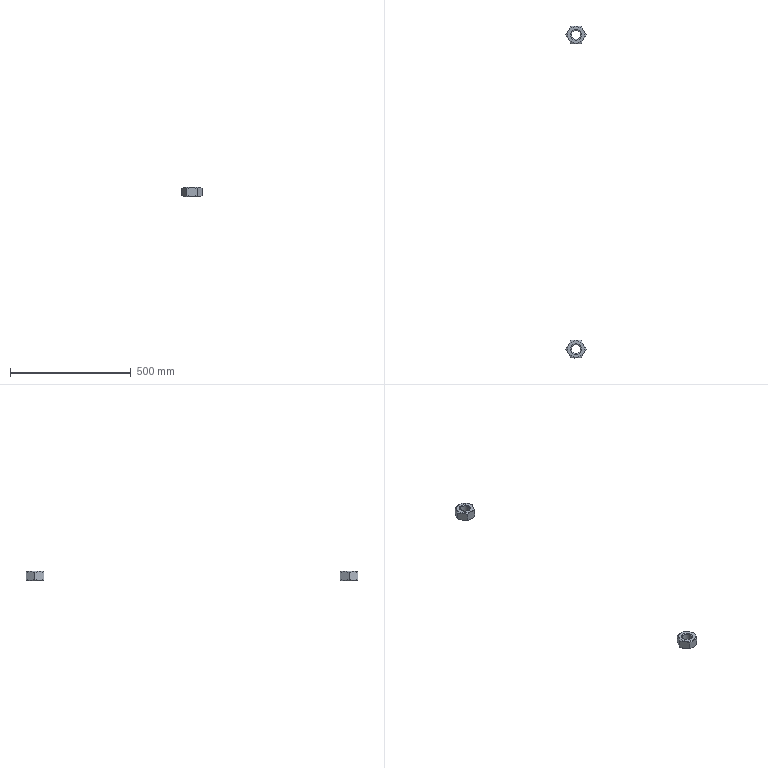Part | NX | features 11.SLDPRT 2, Delete Body 1, LINKED_BODY 1, SCALE 1 | 2 solids | 26 faces | box 84.437 x 1373 x 38.25 mm | volume 263240 mm3 | plane 16 | cone 8 | cylinder 2 | commonest cylinder face diameters 37.389 x2
STEP:
#1=CARTESIAN_POINT('',(28.359,882.042,-396.441));
#2=VERTEX_POINT('',#1);
#3=CARTESIAN_POINT('',(49.469,918.604,-396.441));
#4=VERTEX_POINT('',#3);
#5=CARTESIAN_POINT('',(28.359,882.042,-396.441));
#6=CARTESIAN_POINT('',(30.083,885.027,-395.446));
#7=CARTESIAN_POINT('',(33.551,891.033,-393.805));
#8=CARTESIAN_POINT('',(38.885,900.273,-392.862));
#9=CARTESIAN_POINT('',(44.273,909.605,-393.798));
#10=CARTESIAN_POINT('',(47.743,915.616,-395.445));
#11=CARTESIAN_POINT('',(49.469,918.604,-396.441));
#12=B_SPLINE_CURVE_WITH_KNOTS('',3,(#5,#6,#7,#8,#9,#10,#11),.UNSPECIFIED.,.F.,.F.,(4,1,1,1,4),(0.000001339,0.01066,0.02132,0.03198,0.04264),.UNSPECIFIED.);
#13=EDGE_CURVE('',#2,#4,#12,.T.);
#14=ORIENTED_EDGE('',*,*,#13,.F.);
#15=CARTESIAN_POINT('',(28.359,882.042,-425.724));
#16=VERTEX_POINT('',#15);
#17=CARTESIAN_POINT('',(28.359,882.042,-430.207));
#18=DIRECTION('',(0.,0.,1.));
#19=VECTOR('',#18,1000.);
#20=LINE('',#17,#19);
#21=EDGE_CURVE('',#16,#2,#20,.T.);
#22=ORIENTED_EDGE('',*,*,#21,.F.);
#23=CARTESIAN_POINT('',(49.469,918.604,-425.724));
#24=VERTEX_POINT('',#23);
#25=CARTESIAN_POINT('',(49.469,918.604,-425.724));
#26=CARTESIAN_POINT('',(47.745,915.619,-426.719));
#27=CARTESIAN_POINT('',(44.277,909.613,-428.36));
#28=CARTESIAN_POINT('',(38.943,900.373,-429.303));
#29=CARTESIAN_POINT('',(33.555,891.042,-428.367));
#30=CARTESIAN_POINT('',(30.085,885.031,-426.72));
#31=CARTESIAN_POINT('',(28.359,882.042,-425.724));
#32=B_SPLINE_CURVE_WITH_KNOTS('',3,(#25,#26,#27,#28,#29,#30,#31),.UNSPECIFIED.,.F.,.F.,(4,1,1,1,4),(0.000001339,0.01066,0.02132,0.03198,0.04264),.UNSPECIFIED.);
#33=EDGE_CURVE('',#24,#16,#32,.T.);
#34=ORIENTED_EDGE('',*,*,#33,.F.);
#35=CARTESIAN_POINT('',(49.469,918.604,-430.207));
#36=DIRECTION('',(0.,0.,1.));
#37=VECTOR('',#36,1000.);
#38=LINE('',#35,#37);
#39=EDGE_CURVE('',#24,#4,#38,.T.);
#40=ORIENTED_EDGE('',*,*,#39,.T.);
#41=EDGE_LOOP('',(#14,#22,#34,#40));
#42=FACE_BOUND('',#41,.T.);
#43=CARTESIAN_POINT('',(28.359,882.042,-430.207));
#44=DIRECTION('',(0.866,-0.5,0.));
#45=DIRECTION('',(0.5,0.866,0.));
#46=AXIS2_PLACEMENT_3D('',#43,#44,#45);
#47=PLANE('',#46);
#48=ADVANCED_FACE('',(#42),#47,.T.);
#49=CARTESIAN_POINT('',(-13.859,882.042,-396.441));
#50=VERTEX_POINT('',#49);
#51=CARTESIAN_POINT('',(-13.859,882.042,-396.441));
#52=CARTESIAN_POINT('',(-10.426,882.042,-395.45));
#53=CARTESIAN_POINT('',(-3.394,882.042,-393.789));
#54=CARTESIAN_POINT('',(7.222,882.042,-392.864));
#55=CARTESIAN_POINT('',(18.042,882.042,-393.809));
#56=CARTESIAN_POINT('',(24.947,882.042,-395.456));
#57=CARTESIAN_POINT('',(28.359,882.042,-396.441));
#58=B_SPLINE_CURVE_WITH_KNOTS('',3,(#51,#52,#53,#54,#55,#56,#57),.UNSPECIFIED.,.F.,.F.,(4,1,1,1,4),(0.03747,0.04815,0.05883,0.06951,0.08019),.UNSPECIFIED.);
#59=EDGE_CURVE('',#50,#2,#58,.T.);
#60=ORIENTED_EDGE('',*,*,#59,.F.);
#61=CARTESIAN_POINT('',(-13.859,882.042,-425.724));
#62=VERTEX_POINT('',#61);
#63=CARTESIAN_POINT('',(-13.859,882.042,-430.207));
#64=DIRECTION('',(0.,0.,1.));
#65=VECTOR('',#64,1000.);
#66=LINE('',#63,#65);
#67=EDGE_CURVE('',#62,#50,#66,.T.);
#68=ORIENTED_EDGE('',*,*,#67,.F.);
#69=CARTESIAN_POINT('',(-13.859,882.042,-425.724));
#70=CARTESIAN_POINT('',(-10.426,882.042,-426.715));
#71=CARTESIAN_POINT('',(-3.394,882.042,-428.376));
#72=CARTESIAN_POINT('',(7.222,882.042,-429.301));
#73=CARTESIAN_POINT('',(18.042,882.042,-428.356));
#74=CARTESIAN_POINT('',(24.947,882.042,-426.709));
#75=CARTESIAN_POINT('',(28.359,882.042,-425.724));
#76=B_SPLINE_CURVE_WITH_KNOTS('',3,(#69,#70,#71,#72,#73,#74,#75),.UNSPECIFIED.,.F.,.F.,(4,1,1,1,4),(0.03747,0.04815,0.05883,0.06951,0.08019),.UNSPECIFIED.);
#77=EDGE_CURVE('',#16,#62,#76,.F.);
#78=ORIENTED_EDGE('',*,*,#77,.F.);
#79=ORIENTED_EDGE('',*,*,#21,.T.);
#80=EDGE_LOOP('',(#60,#68,#78,#79));
#81=FACE_BOUND('',#80,.T.);
#82=CARTESIAN_POINT('',(-13.859,882.042,-430.207));
#83=DIRECTION('',(0.,-1.,0.));
#84=DIRECTION('',(1.,0.,0.));
#85=AXIS2_PLACEMENT_3D('',#82,#83,#84);
#86=PLANE('',#85);
#87=ADVANCED_FACE('',(#81),#86,.T.);
#88=CARTESIAN_POINT('',(-34.969,918.604,-396.441));
#89=VERTEX_POINT('',#88);
#90=CARTESIAN_POINT('',(-34.969,918.604,-396.441));
#91=CARTESIAN_POINT('',(-33.245,915.619,-395.446));
#92=CARTESIAN_POINT('',(-29.777,909.613,-393.805));
#93=CARTESIAN_POINT('',(-24.443,900.373,-392.862));
#94=CARTESIAN_POINT('',(-19.055,891.042,-393.798));
#95=CARTESIAN_POINT('',(-15.585,885.031,-395.445));
#96=CARTESIAN_POINT('',(-13.859,882.042,-396.441));
#97=B_SPLINE_CURVE_WITH_KNOTS('',3,(#90,#91,#92,#93,#94,#95,#96),.UNSPECIFIED.,.F.,.F.,(4,1,1,1,4),(0.000001339,0.01066,0.02132,0.03198,0.04264),.UNSPECIFIED.);
#98=EDGE_CURVE('',#89,#50,#97,.T.);
#99=ORIENTED_EDGE('',*,*,#98,.F.);
#100=CARTESIAN_POINT('',(-34.969,918.604,-425.724));
#101=VERTEX_POINT('',#100);
#102=CARTESIAN_POINT('',(-34.969,918.604,-430.207));
#103=DIRECTION('',(0.,0.,1.));
#104=VECTOR('',#103,1000.);
#105=LINE('',#102,#104);
#106=EDGE_CURVE('',#101,#89,#105,.T.);
#107=ORIENTED_EDGE('',*,*,#106,.F.);
#108=CARTESIAN_POINT('',(-13.859,882.042,-425.724));
#109=CARTESIAN_POINT('',(-15.583,885.027,-426.719));
#110=CARTESIAN_POINT('',(-19.051,891.033,-428.36));
#111=CARTESIAN_POINT('',(-24.385,900.273,-429.303));
#112=CARTESIAN_POINT('',(-29.773,909.605,-428.367));
#113=CARTESIAN_POINT('',(-33.243,915.616,-426.72));
#114=CARTESIAN_POINT('',(-34.969,918.604,-425.724));
#115=B_SPLINE_CURVE_WITH_KNOTS('',3,(#108,#109,#110,#111,#112,#113,#114),.UNSPECIFIED.,.F.,.F.,(4,1,1,1,4),(0.000001339,0.01066,0.02132,0.03198,0.04264),.UNSPECIFIED.);
#116=EDGE_CURVE('',#62,#101,#115,.T.);
#117=ORIENTED_EDGE('',*,*,#116,.F.);
#118=ORIENTED_EDGE('',*,*,#67,.T.);
#119=EDGE_LOOP('',(#99,#107,#117,#118));
#120=FACE_BOUND('',#119,.T.);
#121=CARTESIAN_POINT('',(-34.969,918.604,-430.207));
#122=DIRECTION('',(-0.866,-0.5,0.));
#123=DIRECTION('',(0.5,-0.866,0.));
#124=AXIS2_PLACEMENT_3D('',#121,#122,#123);
#125=PLANE('',#124);
#126=ADVANCED_FACE('',(#120),#125,.T.);
#127=CARTESIAN_POINT('',(-13.859,955.167,-396.441));
#128=VERTEX_POINT('',#127);
#129=CARTESIAN_POINT('',(-13.859,955.167,-396.441));
#130=CARTESIAN_POINT('',(-15.583,952.182,-395.446));
#131=CARTESIAN_POINT('',(-19.051,946.175,-393.805));
#132=CARTESIAN_POINT('',(-24.385,936.936,-392.862));
#133=CARTESIAN_POINT('',(-29.773,927.604,-393.798));
#134=CARTESIAN_POINT('',(-33.243,921.593,-395.445));
#135=CARTESIAN_POINT('',(-34.969,918.604,-396.441));
#136=B_SPLINE_CURVE_WITH_KNOTS('',3,(#129,#130,#131,#132,#133,#134,#135),.UNSPECIFIED.,.F.,.F.,(4,1,1,1,4),(0.000001339,0.01066,0.02132,0.03198,0.04264),.UNSPECIFIED.);
#137=EDGE_CURVE('',#128,#89,#136,.T.);
#138=ORIENTED_EDGE('',*,*,#137,.F.);
#139=CARTESIAN_POINT('',(-13.859,955.167,-425.724));
#140=VERTEX_POINT('',#139);
#141=CARTESIAN_POINT('',(-13.859,955.167,-430.207));
#142=DIRECTION('',(0.,0.,1.));
#143=VECTOR('',#142,1000.);
#144=LINE('',#141,#143);
#145=EDGE_CURVE('',#140,#128,#144,.T.);
#146=ORIENTED_EDGE('',*,*,#145,.F.);
#147=CARTESIAN_POINT('',(-34.969,918.604,-425.724));
#148=CARTESIAN_POINT('',(-33.245,921.589,-426.719));
#149=CARTESIAN_POINT('',(-29.777,927.596,-428.36));
#150=CARTESIAN_POINT('',(-24.443,936.835,-429.303));
#151=CARTESIAN_POINT('',(-19.055,946.167,-428.367));
#152=CARTESIAN_POINT('',(-15.585,952.178,-426.72));
#153=CARTESIAN_POINT('',(-13.859,955.167,-425.724));
#154=B_SPLINE_CURVE_WITH_KNOTS('',3,(#147,#148,#149,#150,#151,#152,#153),.UNSPECIFIED.,.F.,.F.,(4,1,1,1,4),(0.000001339,0.01066,0.02132,0.03198,0.04264),.UNSPECIFIED.);
#155=EDGE_CURVE('',#101,#140,#154,.T.);
#156=ORIENTED_EDGE('',*,*,#155,.F.);
#157=ORIENTED_EDGE('',*,*,#106,.T.);
#158=EDGE_LOOP('',(#138,#146,#156,#157));
#159=FACE_BOUND('',#158,.T.);
#160=CARTESIAN_POINT('',(-13.859,955.167,-430.207));
#161=DIRECTION('',(-0.866,0.5,0.));
#162=DIRECTION('',(-0.5,-0.866,0.));
#163=AXIS2_PLACEMENT_3D('',#160,#161,#162);
#164=PLANE('',#163);
#165=ADVANCED_FACE('',(#159),#164,.T.);
#166=CARTESIAN_POINT('',(28.359,955.167,-396.441));
#167=VERTEX_POINT('',#166);
#168=CARTESIAN_POINT('',(-13.859,955.167,-396.441));
#169=CARTESIAN_POINT('',(-10.426,955.167,-395.45));
#170=CARTESIAN_POINT('',(-3.394,955.167,-393.789));
#171=CARTESIAN_POINT('',(7.222,955.167,-392.864));
#172=CARTESIAN_POINT('',(18.042,955.167,-393.809));
#173=CARTESIAN_POINT('',(24.947,955.167,-395.456));
#174=CARTESIAN_POINT('',(28.359,955.167,-396.441));
#175=B_SPLINE_CURVE_WITH_KNOTS('',3,(#168,#169,#170,#171,#172,#173,#174),.UNSPECIFIED.,.F.,.F.,(4,1,1,1,4),(0.03747,0.04815,0.05883,0.06951,0.08019),.UNSPECIFIED.);
#176=EDGE_CURVE('',#167,#128,#175,.F.);
#177=ORIENTED_EDGE('',*,*,#176,.F.);
#178=CARTESIAN_POINT('',(28.359,955.167,-425.724));
#179=VERTEX_POINT('',#178);
#180=CARTESIAN_POINT('',(28.359,955.167,-430.207));
#181=DIRECTION('',(0.,0.,1.));
#182=VECTOR('',#181,1000.);
#183=LINE('',#180,#182);
#184=EDGE_CURVE('',#179,#167,#183,.T.);
#185=ORIENTED_EDGE('',*,*,#184,.F.);
#186=CARTESIAN_POINT('',(-13.859,955.167,-425.724));
#187=CARTESIAN_POINT('',(-10.426,955.167,-426.715));
#188=CARTESIAN_POINT('',(-3.394,955.167,-428.376));
#189=CARTESIAN_POINT('',(7.222,955.167,-429.301));
#190=CARTESIAN_POINT('',(18.042,955.167,-428.356));
#191=CARTESIAN_POINT('',(24.947,955.167,-426.709));
#192=CARTESIAN_POINT('',(28.359,955.167,-425.724));
#193=B_SPLINE_CURVE_WITH_KNOTS('',3,(#186,#187,#188,#189,#190,#191,#192),.UNSPECIFIED.,.F.,.F.,(4,1,1,1,4),(0.03747,0.04815,0.05883,0.06951,0.08019),.UNSPECIFIED.);
#194=EDGE_CURVE('',#140,#179,#193,.T.);
#195=ORIENTED_EDGE('',*,*,#194,.F.);
#196=ORIENTED_EDGE('',*,*,#145,.T.);
#197=EDGE_LOOP('',(#177,#185,#195,#196));
#198=FACE_BOUND('',#197,.T.);
#199=CARTESIAN_POINT('',(28.359,955.167,-430.207));
#200=DIRECTION('',(0.,1.,0.));
#201=DIRECTION('',(0.,0.,1.));
#202=AXIS2_PLACEMENT_3D('',#199,#200,#201);
#203=PLANE('',#202);
#204=ADVANCED_FACE('',(#198),#203,.T.);
#205=CARTESIAN_POINT('',(49.469,918.604,-396.441));
#206=CARTESIAN_POINT('',(47.745,921.589,-395.446));
#207=CARTESIAN_POINT('',(44.277,927.596,-393.805));
#208=CARTESIAN_POINT('',(38.943,936.835,-392.862));
#209=CARTESIAN_POINT('',(33.555,946.167,-393.798));
#210=CARTESIAN_POINT('',(30.085,952.178,-395.445));
#211=CARTESIAN_POINT('',(28.359,955.167,-396.441));
#212=B_SPLINE_CURVE_WITH_KNOTS('',3,(#205,#206,#207,#208,#209,#210,#211),.UNSPECIFIED.,.F.,.F.,(4,1,1,1,4),(0.000001339,0.01066,0.02132,0.03198,0.04264),.UNSPECIFIED.);
#213=EDGE_CURVE('',#4,#167,#212,.T.);
#214=ORIENTED_EDGE('',*,*,#213,.F.);
#215=ORIENTED_EDGE('',*,*,#39,.F.);
#216=CARTESIAN_POINT('',(28.359,955.167,-425.724));
#217=CARTESIAN_POINT('',(30.083,952.182,-426.719));
#218=CARTESIAN_POINT('',(33.551,946.175,-428.36));
#219=CARTESIAN_POINT('',(38.885,936.936,-429.303));
#220=CARTESIAN_POINT('',(44.273,927.604,-428.367));
#221=CARTESIAN_POINT('',(47.743,921.593,-426.72));
#222=CARTESIAN_POINT('',(49.469,918.604,-425.724));
#223=B_SPLINE_CURVE_WITH_KNOTS('',3,(#216,#217,#218,#219,#220,#221,#222),.UNSPECIFIED.,.F.,.F.,(4,1,1,1,4),(0.000001339,0.01066,0.02132,0.03198,0.04264),.UNSPECIFIED.);
#224=EDGE_CURVE('',#179,#24,#223,.T.);
#225=ORIENTED_EDGE('',*,*,#224,.F.);
#226=ORIENTED_EDGE('',*,*,#184,.T.);
#227=EDGE_LOOP('',(#214,#215,#225,#226));
#228=FACE_BOUND('',#227,.T.);
#229=CARTESIAN_POINT('',(49.469,918.604,-430.207));
#230=DIRECTION('',(0.866,0.5,0.));
#231=DIRECTION('',(-0.5,0.866,0.));
#232=AXIS2_PLACEMENT_3D('',#229,#230,#231);
#233=PLANE('',#232);
#234=ADVANCED_FACE('',(#228),#233,.T.);
#235=CARTESIAN_POINT('',(28.142,918.604,-430.207));
#236=VERTEX_POINT('',#235);
#237=CARTESIAN_POINT('',(7.25,918.604,-430.207));
#238=DIRECTION('',(0.,0.,1.));
#239=DIRECTION('',(1.,0.,0.));
#240=AXIS2_PLACEMENT_3D('',#237,#238,#239);
#241=CIRCLE('',#240,20.892);
#242=EDGE_CURVE('',#236,#236,#241,.T.);
#243=ORIENTED_EDGE('',*,*,#242,.T.);
#244=EDGE_LOOP('',(#243));
#245=FACE_BOUND('',#244,.T.);
#246=CARTESIAN_POINT('',(-27.203,918.604,-430.207));
#247=VERTEX_POINT('',#246);
#248=CARTESIAN_POINT('',(7.25,918.604,-430.207));
#249=DIRECTION('',(0.,0.,-1.));
#250=DIRECTION('',(-1.,0.,0.));
#251=AXIS2_PLACEMENT_3D('',#248,#249,#250);
#252=CIRCLE('',#251,34.453);
#253=EDGE_CURVE('',#247,#247,#252,.T.);
#254=ORIENTED_EDGE('',*,*,#253,.T.);
#255=EDGE_LOOP('',(#254));
#256=FACE_BOUND('',#255,.T.);
#257=CARTESIAN_POINT('',(49.469,918.604,-430.207));
#258=DIRECTION('',(0.,0.,1.));
#259=DIRECTION('',(1.,0.,0.));
#260=AXIS2_PLACEMENT_3D('',#257,#258,#259);
#261=PLANE('',#260);
#262=ADVANCED_FACE('',(#245,#256),#261,.F.);
#263=CARTESIAN_POINT('',(29.75,918.604,-391.957));
#264=VERTEX_POINT('',#263);
#265=CARTESIAN_POINT('',(7.25,918.604,-391.957));
#266=DIRECTION('',(0.,0.,1.));
#267=DIRECTION('',(1.,0.,0.));
#268=AXIS2_PLACEMENT_3D('',#265,#266,#267);
#269=CIRCLE('',#268,22.5);
#270=EDGE_CURVE('',#264,#264,#269,.F.);
#271=ORIENTED_EDGE('',*,*,#270,.T.);
#272=EDGE_LOOP('',(#271));
#273=FACE_BOUND('',#272,.T.);
#274=CARTESIAN_POINT('',(-27.203,918.604,-391.957));
#275=VERTEX_POINT('',#274);
#276=CARTESIAN_POINT('',(7.25,918.604,-391.957));
#277=DIRECTION('',(0.,0.,-1.));
#278=DIRECTION('',(-1.,0.,0.));
#279=AXIS2_PLACEMENT_3D('',#276,#277,#278);
#280=CIRCLE('',#279,34.453);
#281=EDGE_CURVE('',#275,#275,#280,.T.);
#282=ORIENTED_EDGE('',*,*,#281,.F.);
#283=EDGE_LOOP('',(#282));
#284=FACE_BOUND('',#283,.T.);
#285=CARTESIAN_POINT('',(49.469,918.604,-391.957));
#286=DIRECTION('',(0.,0.,1.));
#287=DIRECTION('',(1.,0.,0.));
#288=AXIS2_PLACEMENT_3D('',#285,#286,#287);
#289=PLANE('',#288);
#290=ADVANCED_FACE('',(#273,#284),#289,.T.);
#291=CARTESIAN_POINT('',(25.945,918.604,-426.402));
#292=VERTEX_POINT('',#291);
#293=CARTESIAN_POINT('',(7.25,918.604,-426.402));
#294=DIRECTION('',(0.,0.,1.));
#295=DIRECTION('',(1.,0.,0.));
#296=AXIS2_PLACEMENT_3D('',#293,#294,#295);
#297=CIRCLE('',#296,18.695);
#298=EDGE_CURVE('',#292,#292,#297,.F.);
#299=ORIENTED_EDGE('',*,*,#298,.T.);
#300=EDGE_LOOP('',(#299));
#301=FACE_BOUND('',#300,.T.);
#302=CARTESIAN_POINT('',(25.945,918.604,-394.154));
#303=VERTEX_POINT('',#302);
#304=CARTESIAN_POINT('',(7.25,918.604,-394.154));
#305=DIRECTION('',(0.,0.,1.));
#306=DIRECTION('',(1.,0.,0.));
#307=AXIS2_PLACEMENT_3D('',#304,#305,#306);
#308=CIRCLE('',#307,18.695);
#309=EDGE_CURVE('',#303,#303,#308,.T.);
#310=ORIENTED_EDGE('',*,*,#309,.T.);
#311=EDGE_LOOP('',(#310));
#312=FACE_BOUND('',#311,.T.);
#313=CARTESIAN_POINT('',(7.25,918.604,-430.207));
#314=DIRECTION('',(0.,0.,1.));
#315=DIRECTION('',(1.,0.,0.));
#316=AXIS2_PLACEMENT_3D('',#313,#314,#315);
#317=CYLINDRICAL_SURFACE('',#316,18.695);
#318=ADVANCED_FACE('',(#301,#312),#317,.F.);
#319=ORIENTED_EDGE('',*,*,#33,.T.);
#320=ORIENTED_EDGE('',*,*,#77,.T.);
#321=ORIENTED_EDGE('',*,*,#116,.T.);
#322=ORIENTED_EDGE('',*,*,#155,.T.);
#323=ORIENTED_EDGE('',*,*,#194,.T.);
#324=ORIENTED_EDGE('',*,*,#224,.T.);
#325=EDGE_LOOP('',(#319,#320,#321,#322,#323,#324));
#326=FACE_BOUND('',#325,.T.);
#327=ORIENTED_EDGE('',*,*,#253,.F.);
#328=EDGE_LOOP('',(#327));
#329=FACE_BOUND('',#328,.T.);
#330=CARTESIAN_POINT('',(7.25,918.604,-425.724));
#331=DIRECTION('',(0.,0.,1.));
#332=DIRECTION('',(1.,0.,0.));
#333=AXIS2_PLACEMENT_3D('',#330,#331,#332);
#334=CONICAL_SURFACE('',#333,42.219,1.047);
#335=ADVANCED_FACE('',(#326,#329),#334,.T.);
#336=ORIENTED_EDGE('',*,*,#13,.T.);
#337=ORIENTED_EDGE('',*,*,#213,.T.);
#338=ORIENTED_EDGE('',*,*,#176,.T.);
#339=ORIENTED_EDGE('',*,*,#137,.T.);
#340=ORIENTED_EDGE('',*,*,#98,.T.);
#341=ORIENTED_EDGE('',*,*,#59,.T.);
#342=EDGE_LOOP('',(#336,#337,#338,#339,#340,#341));
#343=FACE_BOUND('',#342,.T.);
#344=ORIENTED_EDGE('',*,*,#281,.T.);
#345=EDGE_LOOP('',(#344));
#346=FACE_BOUND('',#345,.T.);
#347=CARTESIAN_POINT('',(7.25,918.604,-391.957));
#348=DIRECTION('',(0.,0.,-1.));
#349=DIRECTION('',(-1.,0.,0.));
#350=AXIS2_PLACEMENT_3D('',#347,#348,#349);
#351=CONICAL_SURFACE('',#350,34.453,1.047);
#352=ADVANCED_FACE('',(#343,#346),#351,.T.);
#353=ORIENTED_EDGE('',*,*,#298,.F.);
#354=EDGE_LOOP('',(#353));
#355=FACE_BOUND('',#354,.T.);
#356=ORIENTED_EDGE('',*,*,#242,.F.);
#357=EDGE_LOOP('',(#356));
#358=FACE_BOUND('',#357,.T.);
#359=CARTESIAN_POINT('',(7.25,918.604,-430.207));
#360=DIRECTION('',(0.,0.,-1.));
#361=DIRECTION('',(-1.,0.,0.));
#362=AXIS2_PLACEMENT_3D('',#359,#360,#361);
#363=CONICAL_SURFACE('',#362,20.892,0.5236);
#364=ADVANCED_FACE('',(#355,#358),#363,.F.);
#365=ORIENTED_EDGE('',*,*,#270,.F.);
#366=EDGE_LOOP('',(#365));
#367=FACE_BOUND('',#366,.T.);
#368=ORIENTED_EDGE('',*,*,#309,.F.);
#369=EDGE_LOOP('',(#368));
#370=FACE_BOUND('',#369,.T.);
#371=CARTESIAN_POINT('',(7.25,918.604,-394.154));
#372=DIRECTION('',(0.,0.,1.));
#373=DIRECTION('',(1.,0.,0.));
#374=AXIS2_PLACEMENT_3D('',#371,#372,#373);
#375=CONICAL_SURFACE('',#374,18.695,1.047);
#376=ADVANCED_FACE('',(#367,#370),#375,.F.);
#377=CLOSED_SHELL('',(#48,#87,#126,#165,#204,#234,#262,#290,#318,#335,#352,#364,#376));
#378=MANIFOLD_SOLID_BREP('',#377);
#379=CARTESIAN_POINT('',(28.359,2181.417,-396.441));
#380=VERTEX_POINT('',#379);
#381=CARTESIAN_POINT('',(49.469,2217.979,-396.441));
#382=VERTEX_POINT('',#381);
#383=CARTESIAN_POINT('',(28.359,2181.417,-396.441));
#384=CARTESIAN_POINT('',(30.083,2184.402,-395.446));
#385=CARTESIAN_POINT('',(33.551,2190.408,-393.805));
#386=CARTESIAN_POINT('',(38.885,2199.648,-392.862));
#387=CARTESIAN_POINT('',(44.273,2208.98,-393.798));
#388=CARTESIAN_POINT('',(47.743,2214.991,-395.445));
#389=CARTESIAN_POINT('',(49.469,2217.979,-396.441));
#390=B_SPLINE_CURVE_WITH_KNOTS('',3,(#383,#384,#385,#386,#387,#388,#389),.UNSPECIFIED.,.F.,.F.,(4,1,1,1,4),(0.000001339,0.01066,0.02132,0.03198,0.04264),.UNSPECIFIED.);
#391=EDGE_CURVE('',#380,#382,#390,.T.);
#392=ORIENTED_EDGE('',*,*,#391,.F.);
#393=CARTESIAN_POINT('',(28.359,2181.417,-425.724));
#394=VERTEX_POINT('',#393);
#395=CARTESIAN_POINT('',(28.359,2181.417,-430.207));
#396=DIRECTION('',(0.,0.,1.));
#397=VECTOR('',#396,1000.);
#398=LINE('',#395,#397);
#399=EDGE_CURVE('',#394,#380,#398,.T.);
#400=ORIENTED_EDGE('',*,*,#399,.F.);
#401=CARTESIAN_POINT('',(49.469,2217.979,-425.724));
#402=VERTEX_POINT('',#401);
#403=CARTESIAN_POINT('',(49.469,2217.979,-425.724));
#404=CARTESIAN_POINT('',(47.745,2214.994,-426.719));
#405=CARTESIAN_POINT('',(44.277,2208.988,-428.36));
#406=CARTESIAN_POINT('',(38.943,2199.748,-429.303));
#407=CARTESIAN_POINT('',(33.555,2190.417,-428.367));
#408=CARTESIAN_POINT('',(30.085,2184.406,-426.72));
#409=CARTESIAN_POINT('',(28.359,2181.417,-425.724));
#410=B_SPLINE_CURVE_WITH_KNOTS('',3,(#403,#404,#405,#406,#407,#408,#409),.UNSPECIFIED.,.F.,.F.,(4,1,1,1,4),(0.000001339,0.01066,0.02132,0.03198,0.04264),.UNSPECIFIED.);
#411=EDGE_CURVE('',#402,#394,#410,.T.);
#412=ORIENTED_EDGE('',*,*,#411,.F.);
#413=CARTESIAN_POINT('',(49.469,2217.979,-430.207));
#414=DIRECTION('',(0.,0.,1.));
#415=VECTOR('',#414,1000.);
#416=LINE('',#413,#415);
#417=EDGE_CURVE('',#402,#382,#416,.T.);
#418=ORIENTED_EDGE('',*,*,#417,.T.);
#419=EDGE_LOOP('',(#392,#400,#412,#418));
#420=FACE_BOUND('',#419,.T.);
#421=CARTESIAN_POINT('',(28.359,2181.417,-430.207));
#422=DIRECTION('',(0.866,-0.5,0.));
#423=DIRECTION('',(0.5,0.866,0.));
#424=AXIS2_PLACEMENT_3D('',#421,#422,#423);
#425=PLANE('',#424);
#426=ADVANCED_FACE('',(#420),#425,.T.);
#427=CARTESIAN_POINT('',(-13.859,2181.417,-396.441));
#428=VERTEX_POINT('',#427);
#429=CARTESIAN_POINT('',(-13.859,2181.417,-396.441));
#430=CARTESIAN_POINT('',(-10.426,2181.417,-395.45));
#431=CARTESIAN_POINT('',(-3.394,2181.417,-393.789));
#432=CARTESIAN_POINT('',(7.222,2181.417,-392.864));
#433=CARTESIAN_POINT('',(18.042,2181.417,-393.809));
#434=CARTESIAN_POINT('',(24.947,2181.417,-395.456));
#435=CARTESIAN_POINT('',(28.359,2181.417,-396.441));
#436=B_SPLINE_CURVE_WITH_KNOTS('',3,(#429,#430,#431,#432,#433,#434,#435),.UNSPECIFIED.,.F.,.F.,(4,1,1,1,4),(0.03747,0.04815,0.05883,0.06951,0.08019),.UNSPECIFIED.);
#437=EDGE_CURVE('',#428,#380,#436,.T.);
#438=ORIENTED_EDGE('',*,*,#437,.F.);
#439=CARTESIAN_POINT('',(-13.859,2181.417,-425.724));
#440=VERTEX_POINT('',#439);
#441=CARTESIAN_POINT('',(-13.859,2181.417,-430.207));
#442=DIRECTION('',(0.,0.,1.));
#443=VECTOR('',#442,1000.);
#444=LINE('',#441,#443);
#445=EDGE_CURVE('',#440,#428,#444,.T.);
#446=ORIENTED_EDGE('',*,*,#445,.F.);
#447=CARTESIAN_POINT('',(-13.859,2181.417,-425.724));
#448=CARTESIAN_POINT('',(-10.426,2181.417,-426.715));
#449=CARTESIAN_POINT('',(-3.394,2181.417,-428.376));
#450=CARTESIAN_POINT('',(7.222,2181.417,-429.301));
#451=CARTESIAN_POINT('',(18.042,2181.417,-428.356));
#452=CARTESIAN_POINT('',(24.947,2181.417,-426.709));
#453=CARTESIAN_POINT('',(28.359,2181.417,-425.724));
#454=B_SPLINE_CURVE_WITH_KNOTS('',3,(#447,#448,#449,#450,#451,#452,#453),.UNSPECIFIED.,.F.,.F.,(4,1,1,1,4),(0.03747,0.04815,0.05883,0.06951,0.08019),.UNSPECIFIED.);
#455=EDGE_CURVE('',#394,#440,#454,.F.);
#456=ORIENTED_EDGE('',*,*,#455,.F.);
#457=ORIENTED_EDGE('',*,*,#399,.T.);
#458=EDGE_LOOP('',(#438,#446,#456,#457));
#459=FACE_BOUND('',#458,.T.);
#460=CARTESIAN_POINT('',(-13.859,2181.417,-430.207));
#461=DIRECTION('',(0.,-1.,0.));
#462=DIRECTION('',(1.,0.,0.));
#463=AXIS2_PLACEMENT_3D('',#460,#461,#462);
#464=PLANE('',#463);
#465=ADVANCED_FACE('',(#459),#464,.T.);
#466=CARTESIAN_POINT('',(-34.969,2217.979,-396.441));
#467=VERTEX_POINT('',#466);
#468=CARTESIAN_POINT('',(-34.969,2217.979,-396.441));
#469=CARTESIAN_POINT('',(-33.245,2214.994,-395.446));
#470=CARTESIAN_POINT('',(-29.777,2208.988,-393.805));
#471=CARTESIAN_POINT('',(-24.443,2199.748,-392.862));
#472=CARTESIAN_POINT('',(-19.055,2190.417,-393.798));
#473=CARTESIAN_POINT('',(-15.585,2184.406,-395.445));
#474=CARTESIAN_POINT('',(-13.859,2181.417,-396.441));
#475=B_SPLINE_CURVE_WITH_KNOTS('',3,(#468,#469,#470,#471,#472,#473,#474),.UNSPECIFIED.,.F.,.F.,(4,1,1,1,4),(0.000001339,0.01066,0.02132,0.03198,0.04264),.UNSPECIFIED.);
#476=EDGE_CURVE('',#467,#428,#475,.T.);
#477=ORIENTED_EDGE('',*,*,#476,.F.);
#478=CARTESIAN_POINT('',(-34.969,2217.979,-425.724));
#479=VERTEX_POINT('',#478);
#480=CARTESIAN_POINT('',(-34.969,2217.979,-430.207));
#481=DIRECTION('',(0.,0.,1.));
#482=VECTOR('',#481,1000.);
#483=LINE('',#480,#482);
#484=EDGE_CURVE('',#479,#467,#483,.T.);
#485=ORIENTED_EDGE('',*,*,#484,.F.);
#486=CARTESIAN_POINT('',(-13.859,2181.417,-425.724));
#487=CARTESIAN_POINT('',(-15.583,2184.402,-426.719));
#488=CARTESIAN_POINT('',(-19.051,2190.408,-428.36));
#489=CARTESIAN_POINT('',(-24.385,2199.648,-429.303));
#490=CARTESIAN_POINT('',(-29.773,2208.98,-428.367));
#491=CARTESIAN_POINT('',(-33.243,2214.991,-426.72));
#492=CARTESIAN_POINT('',(-34.969,2217.979,-425.724));
#493=B_SPLINE_CURVE_WITH_KNOTS('',3,(#486,#487,#488,#489,#490,#491,#492),.UNSPECIFIED.,.F.,.F.,(4,1,1,1,4),(0.000001339,0.01066,0.02132,0.03198,0.04264),.UNSPECIFIED.);
#494=EDGE_CURVE('',#440,#479,#493,.T.);
#495=ORIENTED_EDGE('',*,*,#494,.F.);
#496=ORIENTED_EDGE('',*,*,#445,.T.);
#497=EDGE_LOOP('',(#477,#485,#495,#496));
#498=FACE_BOUND('',#497,.T.);
#499=CARTESIAN_POINT('',(-34.969,2217.979,-430.207));
#500=DIRECTION('',(-0.866,-0.5,0.));
#501=DIRECTION('',(0.5,-0.866,0.));
#502=AXIS2_PLACEMENT_3D('',#499,#500,#501);
#503=PLANE('',#502);
#504=ADVANCED_FACE('',(#498),#503,.T.);
#505=CARTESIAN_POINT('',(-13.859,2254.542,-396.441));
#506=VERTEX_POINT('',#505);
#507=CARTESIAN_POINT('',(-13.859,2254.542,-396.441));
#508=CARTESIAN_POINT('',(-15.583,2251.557,-395.446));
#509=CARTESIAN_POINT('',(-19.051,2245.55,-393.805));
#510=CARTESIAN_POINT('',(-24.385,2236.311,-392.862));
#511=CARTESIAN_POINT('',(-29.773,2226.979,-393.798));
#512=CARTESIAN_POINT('',(-33.243,2220.968,-395.445));
#513=CARTESIAN_POINT('',(-34.969,2217.979,-396.441));
#514=B_SPLINE_CURVE_WITH_KNOTS('',3,(#507,#508,#509,#510,#511,#512,#513),.UNSPECIFIED.,.F.,.F.,(4,1,1,1,4),(0.000001339,0.01066,0.02132,0.03198,0.04264),.UNSPECIFIED.);
#515=EDGE_CURVE('',#506,#467,#514,.T.);
#516=ORIENTED_EDGE('',*,*,#515,.F.);
#517=CARTESIAN_POINT('',(-13.859,2254.542,-425.724));
#518=VERTEX_POINT('',#517);
#519=CARTESIAN_POINT('',(-13.859,2254.542,-430.207));
#520=DIRECTION('',(0.,0.,1.));
#521=VECTOR('',#520,1000.);
#522=LINE('',#519,#521);
#523=EDGE_CURVE('',#518,#506,#522,.T.);
#524=ORIENTED_EDGE('',*,*,#523,.F.);
#525=CARTESIAN_POINT('',(-34.969,2217.979,-425.724));
#526=CARTESIAN_POINT('',(-33.245,2220.964,-426.719));
#527=CARTESIAN_POINT('',(-29.777,2226.971,-428.36));
#528=CARTESIAN_POINT('',(-24.443,2236.21,-429.303));
#529=CARTESIAN_POINT('',(-19.055,2245.542,-428.367));
#530=CARTESIAN_POINT('',(-15.585,2251.553,-426.72));
#531=CARTESIAN_POINT('',(-13.859,2254.542,-425.724));
#532=B_SPLINE_CURVE_WITH_KNOTS('',3,(#525,#526,#527,#528,#529,#530,#531),.UNSPECIFIED.,.F.,.F.,(4,1,1,1,4),(0.000001339,0.01066,0.02132,0.03198,0.04264),.UNSPECIFIED.);
#533=EDGE_CURVE('',#479,#518,#532,.T.);
#534=ORIENTED_EDGE('',*,*,#533,.F.);
#535=ORIENTED_EDGE('',*,*,#484,.T.);
#536=EDGE_LOOP('',(#516,#524,#534,#535));
#537=FACE_BOUND('',#536,.T.);
#538=CARTESIAN_POINT('',(-13.859,2254.542,-430.207));
#539=DIRECTION('',(-0.866,0.5,0.));
#540=DIRECTION('',(-0.5,-0.866,0.));
#541=AXIS2_PLACEMENT_3D('',#538,#539,#540);
#542=PLANE('',#541);
#543=ADVANCED_FACE('',(#537),#542,.T.);
#544=CARTESIAN_POINT('',(28.359,2254.542,-396.441));
#545=VERTEX_POINT('',#544);
#546=CARTESIAN_POINT('',(-13.859,2254.542,-396.441));
#547=CARTESIAN_POINT('',(-10.426,2254.542,-395.45));
#548=CARTESIAN_POINT('',(-3.394,2254.542,-393.789));
#549=CARTESIAN_POINT('',(7.222,2254.542,-392.864));
#550=CARTESIAN_POINT('',(18.042,2254.542,-393.809));
#551=CARTESIAN_POINT('',(24.947,2254.542,-395.456));
#552=CARTESIAN_POINT('',(28.359,2254.542,-396.441));
#553=B_SPLINE_CURVE_WITH_KNOTS('',3,(#546,#547,#548,#549,#550,#551,#552),.UNSPECIFIED.,.F.,.F.,(4,1,1,1,4),(0.03747,0.04815,0.05883,0.06951,0.08019),.UNSPECIFIED.);
#554=EDGE_CURVE('',#545,#506,#553,.F.);
#555=ORIENTED_EDGE('',*,*,#554,.F.);
#556=CARTESIAN_POINT('',(28.359,2254.542,-425.724));
#557=VERTEX_POINT('',#556);
#558=CARTESIAN_POINT('',(28.359,2254.542,-430.207));
#559=DIRECTION('',(0.,0.,1.));
#560=VECTOR('',#559,1000.);
#561=LINE('',#558,#560);
#562=EDGE_CURVE('',#557,#545,#561,.T.);
#563=ORIENTED_EDGE('',*,*,#562,.F.);
#564=CARTESIAN_POINT('',(-13.859,2254.542,-425.724));
#565=CARTESIAN_POINT('',(-10.426,2254.542,-426.715));
#566=CARTESIAN_POINT('',(-3.394,2254.542,-428.376));
#567=CARTESIAN_POINT('',(7.222,2254.542,-429.301));
#568=CARTESIAN_POINT('',(18.042,2254.542,-428.356));
#569=CARTESIAN_POINT('',(24.947,2254.542,-426.709));
#570=CARTESIAN_POINT('',(28.359,2254.542,-425.724));
#571=B_SPLINE_CURVE_WITH_KNOTS('',3,(#564,#565,#566,#567,#568,#569,#570),.UNSPECIFIED.,.F.,.F.,(4,1,1,1,4),(0.03747,0.04815,0.05883,0.06951,0.08019),.UNSPECIFIED.);
#572=EDGE_CURVE('',#518,#557,#571,.T.);
#573=ORIENTED_EDGE('',*,*,#572,.F.);
#574=ORIENTED_EDGE('',*,*,#523,.T.);
#575=EDGE_LOOP('',(#555,#563,#573,#574));
#576=FACE_BOUND('',#575,.T.);
#577=CARTESIAN_POINT('',(28.359,2254.542,-430.207));
#578=DIRECTION('',(0.,1.,0.));
#579=DIRECTION('',(0.,0.,1.));
#580=AXIS2_PLACEMENT_3D('',#577,#578,#579);
#581=PLANE('',#580);
#582=ADVANCED_FACE('',(#576),#581,.T.);
#583=CARTESIAN_POINT('',(49.469,2217.979,-396.441));
#584=CARTESIAN_POINT('',(47.745,2220.964,-395.446));
#585=CARTESIAN_POINT('',(44.277,2226.971,-393.805));
#586=CARTESIAN_POINT('',(38.943,2236.21,-392.862));
#587=CARTESIAN_POINT('',(33.555,2245.542,-393.798));
#588=CARTESIAN_POINT('',(30.085,2251.553,-395.445));
#589=CARTESIAN_POINT('',(28.359,2254.542,-396.441));
#590=B_SPLINE_CURVE_WITH_KNOTS('',3,(#583,#584,#585,#586,#587,#588,#589),.UNSPECIFIED.,.F.,.F.,(4,1,1,1,4),(0.000001339,0.01066,0.02132,0.03198,0.04264),.UNSPECIFIED.);
#591=EDGE_CURVE('',#382,#545,#590,.T.);
#592=ORIENTED_EDGE('',*,*,#591,.F.);
#593=ORIENTED_EDGE('',*,*,#417,.F.);
#594=CARTESIAN_POINT('',(28.359,2254.542,-425.724));
#595=CARTESIAN_POINT('',(30.083,2251.557,-426.719));
#596=CARTESIAN_POINT('',(33.551,2245.55,-428.36));
#597=CARTESIAN_POINT('',(38.885,2236.311,-429.303));
#598=CARTESIAN_POINT('',(44.273,2226.979,-428.367));
#599=CARTESIAN_POINT('',(47.743,2220.968,-426.72));
#600=CARTESIAN_POINT('',(49.469,2217.979,-425.724));
#601=B_SPLINE_CURVE_WITH_KNOTS('',3,(#594,#595,#596,#597,#598,#599,#600),.UNSPECIFIED.,.F.,.F.,(4,1,1,1,4),(0.000001339,0.01066,0.02132,0.03198,0.04264),.UNSPECIFIED.);
#602=EDGE_CURVE('',#557,#402,#601,.T.);
#603=ORIENTED_EDGE('',*,*,#602,.F.);
#604=ORIENTED_EDGE('',*,*,#562,.T.);
#605=EDGE_LOOP('',(#592,#593,#603,#604));
#606=FACE_BOUND('',#605,.T.);
#607=CARTESIAN_POINT('',(49.469,2217.979,-430.207));
#608=DIRECTION('',(0.866,0.5,0.));
#609=DIRECTION('',(-0.5,0.866,0.));
#610=AXIS2_PLACEMENT_3D('',#607,#608,#609);
#611=PLANE('',#610);
#612=ADVANCED_FACE('',(#606),#611,.T.);
#613=CARTESIAN_POINT('',(28.142,2217.979,-430.207));
#614=VERTEX_POINT('',#613);
#615=CARTESIAN_POINT('',(7.25,2217.979,-430.207));
#616=DIRECTION('',(0.,0.,1.));
#617=DIRECTION('',(1.,0.,0.));
#618=AXIS2_PLACEMENT_3D('',#615,#616,#617);
#619=CIRCLE('',#618,20.892);
#620=EDGE_CURVE('',#614,#614,#619,.T.);
#621=ORIENTED_EDGE('',*,*,#620,.T.);
#622=EDGE_LOOP('',(#621));
#623=FACE_BOUND('',#622,.T.);
#624=CARTESIAN_POINT('',(-27.203,2217.979,-430.207));
#625=VERTEX_POINT('',#624);
#626=CARTESIAN_POINT('',(7.25,2217.979,-430.207));
#627=DIRECTION('',(0.,0.,-1.));
#628=DIRECTION('',(-1.,0.,0.));
#629=AXIS2_PLACEMENT_3D('',#626,#627,#628);
#630=CIRCLE('',#629,34.453);
#631=EDGE_CURVE('',#625,#625,#630,.T.);
#632=ORIENTED_EDGE('',*,*,#631,.T.);
#633=EDGE_LOOP('',(#632));
#634=FACE_BOUND('',#633,.T.);
#635=CARTESIAN_POINT('',(49.469,2217.979,-430.207));
#636=DIRECTION('',(0.,0.,1.));
#637=DIRECTION('',(1.,0.,0.));
#638=AXIS2_PLACEMENT_3D('',#635,#636,#637);
#639=PLANE('',#638);
#640=ADVANCED_FACE('',(#623,#634),#639,.F.);
#641=CARTESIAN_POINT('',(29.75,2217.979,-391.957));
#642=VERTEX_POINT('',#641);
#643=CARTESIAN_POINT('',(7.25,2217.979,-391.957));
#644=DIRECTION('',(0.,0.,1.));
#645=DIRECTION('',(1.,0.,0.));
#646=AXIS2_PLACEMENT_3D('',#643,#644,#645);
#647=CIRCLE('',#646,22.5);
#648=EDGE_CURVE('',#642,#642,#647,.F.);
#649=ORIENTED_EDGE('',*,*,#648,.T.);
#650=EDGE_LOOP('',(#649));
#651=FACE_BOUND('',#650,.T.);
#652=CARTESIAN_POINT('',(-27.203,2217.979,-391.957));
#653=VERTEX_POINT('',#652);
#654=CARTESIAN_POINT('',(7.25,2217.979,-391.957));
#655=DIRECTION('',(0.,0.,-1.));
#656=DIRECTION('',(-1.,0.,0.));
#657=AXIS2_PLACEMENT_3D('',#654,#655,#656);
#658=CIRCLE('',#657,34.453);
#659=EDGE_CURVE('',#653,#653,#658,.T.);
#660=ORIENTED_EDGE('',*,*,#659,.F.);
#661=EDGE_LOOP('',(#660));
#662=FACE_BOUND('',#661,.T.);
#663=CARTESIAN_POINT('',(49.469,2217.979,-391.957));
#664=DIRECTION('',(0.,0.,1.));
#665=DIRECTION('',(1.,0.,0.));
#666=AXIS2_PLACEMENT_3D('',#663,#664,#665);
#667=PLANE('',#666);
#668=ADVANCED_FACE('',(#651,#662),#667,.T.);
#669=CARTESIAN_POINT('',(25.945,2217.979,-426.402));
#670=VERTEX_POINT('',#669);
#671=CARTESIAN_POINT('',(7.25,2217.979,-426.402));
#672=DIRECTION('',(0.,0.,1.));
#673=DIRECTION('',(1.,0.,0.));
#674=AXIS2_PLACEMENT_3D('',#671,#672,#673);
#675=CIRCLE('',#674,18.695);
#676=EDGE_CURVE('',#670,#670,#675,.F.);
#677=ORIENTED_EDGE('',*,*,#676,.T.);
#678=EDGE_LOOP('',(#677));
#679=FACE_BOUND('',#678,.T.);
#680=CARTESIAN_POINT('',(25.945,2217.979,-394.154));
#681=VERTEX_POINT('',#680);
#682=CARTESIAN_POINT('',(7.25,2217.979,-394.154));
#683=DIRECTION('',(0.,0.,1.));
#684=DIRECTION('',(1.,0.,0.));
#685=AXIS2_PLACEMENT_3D('',#682,#683,#684);
#686=CIRCLE('',#685,18.695);
#687=EDGE_CURVE('',#681,#681,#686,.T.);
#688=ORIENTED_EDGE('',*,*,#687,.T.);
#689=EDGE_LOOP('',(#688));
#690=FACE_BOUND('',#689,.T.);
#691=CARTESIAN_POINT('',(7.25,2217.979,-430.207));
#692=DIRECTION('',(0.,0.,1.));
#693=DIRECTION('',(1.,0.,0.));
#694=AXIS2_PLACEMENT_3D('',#691,#692,#693);
#695=CYLINDRICAL_SURFACE('',#694,18.695);
#696=ADVANCED_FACE('',(#679,#690),#695,.F.);
#697=ORIENTED_EDGE('',*,*,#411,.T.);
#698=ORIENTED_EDGE('',*,*,#455,.T.);
#699=ORIENTED_EDGE('',*,*,#494,.T.);
#700=ORIENTED_EDGE('',*,*,#533,.T.);
#701=ORIENTED_EDGE('',*,*,#572,.T.);
#702=ORIENTED_EDGE('',*,*,#602,.T.);
#703=EDGE_LOOP('',(#697,#698,#699,#700,#701,#702));
#704=FACE_BOUND('',#703,.T.);
#705=ORIENTED_EDGE('',*,*,#631,.F.);
#706=EDGE_LOOP('',(#705));
#707=FACE_BOUND('',#706,.T.);
#708=CARTESIAN_POINT('',(7.25,2217.979,-425.724));
#709=DIRECTION('',(0.,0.,1.));
#710=DIRECTION('',(1.,0.,0.));
#711=AXIS2_PLACEMENT_3D('',#708,#709,#710);
#712=CONICAL_SURFACE('',#711,42.219,1.047);
#713=ADVANCED_FACE('',(#704,#707),#712,.T.);
#714=ORIENTED_EDGE('',*,*,#391,.T.);
#715=ORIENTED_EDGE('',*,*,#591,.T.);
#716=ORIENTED_EDGE('',*,*,#554,.T.);
#717=ORIENTED_EDGE('',*,*,#515,.T.);
#718=ORIENTED_EDGE('',*,*,#476,.T.);
#719=ORIENTED_EDGE('',*,*,#437,.T.);
#720=EDGE_LOOP('',(#714,#715,#716,#717,#718,#719));
#721=FACE_BOUND('',#720,.T.);
#722=ORIENTED_EDGE('',*,*,#659,.T.);
#723=EDGE_LOOP('',(#722));
#724=FACE_BOUND('',#723,.T.);
#725=CARTESIAN_POINT('',(7.25,2217.979,-391.957));
#726=DIRECTION('',(0.,0.,-1.));
#727=DIRECTION('',(-1.,0.,0.));
#728=AXIS2_PLACEMENT_3D('',#725,#726,#727);
#729=CONICAL_SURFACE('',#728,34.453,1.047);
#730=ADVANCED_FACE('',(#721,#724),#729,.T.);
#731=ORIENTED_EDGE('',*,*,#676,.F.);
#732=EDGE_LOOP('',(#731));
#733=FACE_BOUND('',#732,.T.);
#734=ORIENTED_EDGE('',*,*,#620,.F.);
#735=EDGE_LOOP('',(#734));
#736=FACE_BOUND('',#735,.T.);
#737=CARTESIAN_POINT('',(7.25,2217.979,-430.207));
#738=DIRECTION('',(0.,0.,-1.));
#739=DIRECTION('',(-1.,0.,0.));
#740=AXIS2_PLACEMENT_3D('',#737,#738,#739);
#741=CONICAL_SURFACE('',#740,20.892,0.5236);
#742=ADVANCED_FACE('',(#733,#736),#741,.F.);
#743=ORIENTED_EDGE('',*,*,#648,.F.);
#744=EDGE_LOOP('',(#743));
#745=FACE_BOUND('',#744,.T.);
#746=ORIENTED_EDGE('',*,*,#687,.F.);
#747=EDGE_LOOP('',(#746));
#748=FACE_BOUND('',#747,.T.);
#749=CARTESIAN_POINT('',(7.25,2217.979,-394.154));
#750=DIRECTION('',(0.,0.,1.));
#751=DIRECTION('',(1.,0.,0.));
#752=AXIS2_PLACEMENT_3D('',#749,#750,#751);
#753=CONICAL_SURFACE('',#752,18.695,1.047);
#754=ADVANCED_FACE('',(#745,#748),#753,.F.);
#755=CLOSED_SHELL('',(#426,#465,#504,#543,#582,#612,#640,#668,#696,#713,#730,#742,#754));
#756=MANIFOLD_SOLID_BREP('',#755);
#757=(LENGTH_UNIT()NAMED_UNIT(*)SI_UNIT(.MILLI.,.METRE.));
#758=UNCERTAINTY_MEASURE_WITH_UNIT(LENGTH_MEASURE(0.0508),#757,'','');
#759=(NAMED_UNIT(*)PLANE_ANGLE_UNIT()SI_UNIT($,.RADIAN.));
#760=(NAMED_UNIT(*)SI_UNIT($,.STERADIAN.)SOLID_ANGLE_UNIT());
#761=(GEOMETRIC_REPRESENTATION_CONTEXT(3)GLOBAL_UNCERTAINTY_ASSIGNED_CONTEXT((#758))GLOBAL_UNIT_ASSIGNED_CONTEXT((#757,#759,#760))REPRESENTATION_CONTEXT('',''));
#762=ADVANCED_BREP_SHAPE_REPRESENTATION('',(#378,#756),#761);